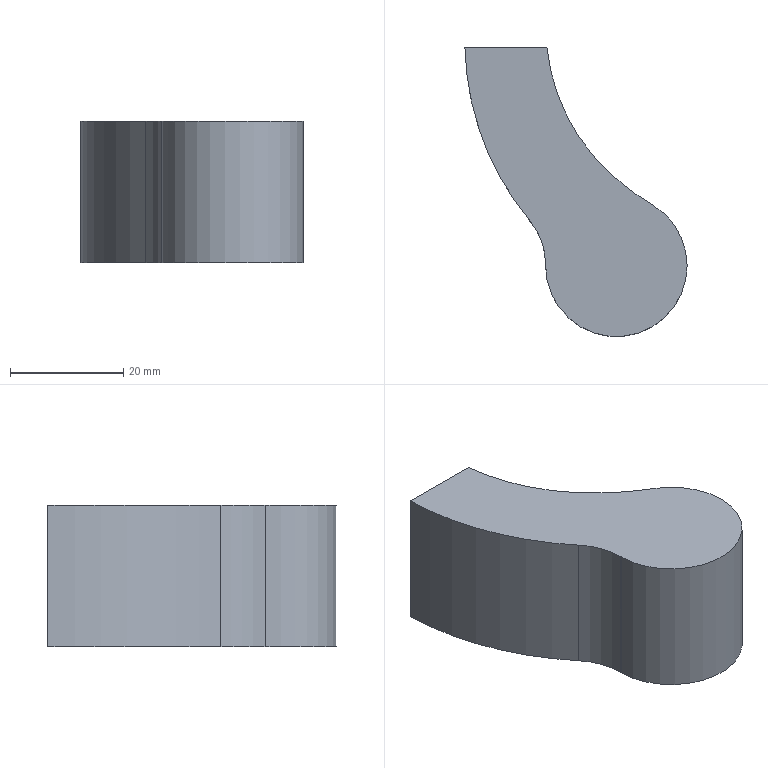Part | SolidWorks | features BaseBody 1 | 1 solid | 19 faces | box 39.25 x 51 x 25 mm | volume 19641 mm3 | cylinder 13 | plane 6 | commonest cylinder face diameters 3.3 x4 25 x3 18 x2 24 x1 70 x1 90 x1
STEP:
#1=CARTESIAN_POINT('',(89.772,84.898,25.));
#2=VERTEX_POINT('',#1);
#3=CARTESIAN_POINT('',(83.667,95.639,25.));
#4=VERTEX_POINT('',#3);
#5=CARTESIAN_POINT('',(77.272,84.898,25.));
#6=DIRECTION('',(0.,0.,1.));
#7=DIRECTION('',(-1.,0.,0.));
#8=AXIS2_PLACEMENT_3D('',#5,#6,#7);
#9=CIRCLE('',#8,12.5);
#10=EDGE_CURVE('',#2,#4,#9,.T.);
#11=ORIENTED_EDGE('',*,*,#10,.F.);
#12=CARTESIAN_POINT('',(89.772,84.898,0.));
#13=VERTEX_POINT('',#12);
#14=CARTESIAN_POINT('',(89.772,84.898,25.));
#15=DIRECTION('',(0.,0.,-1.));
#16=VECTOR('',#15,1000.);
#17=LINE('',#14,#16);
#18=EDGE_CURVE('',#2,#13,#17,.T.);
#19=ORIENTED_EDGE('',*,*,#18,.T.);
#20=CARTESIAN_POINT('',(83.667,95.639,0.));
#21=VERTEX_POINT('',#20);
#22=CARTESIAN_POINT('',(77.272,84.898,0.));
#23=DIRECTION('',(0.,0.,1.));
#24=DIRECTION('',(-1.,0.,0.));
#25=AXIS2_PLACEMENT_3D('',#22,#23,#24);
#26=CIRCLE('',#25,12.5);
#27=EDGE_CURVE('',#13,#21,#26,.T.);
#28=ORIENTED_EDGE('',*,*,#27,.T.);
#29=CARTESIAN_POINT('',(83.667,95.639,25.));
#30=DIRECTION('',(0.,0.,1.));
#31=VECTOR('',#30,1000.);
#32=LINE('',#29,#31);
#33=EDGE_CURVE('',#21,#4,#32,.T.);
#34=ORIENTED_EDGE('',*,*,#33,.T.);
#35=EDGE_LOOP('',(#11,#19,#28,#34));
#36=FACE_OUTER_BOUND('',#35,.T.);
#37=CARTESIAN_POINT('',(77.272,84.898,25.));
#38=DIRECTION('',(0.,0.,-1.));
#39=DIRECTION('',(-1.,0.,0.));
#40=AXIS2_PLACEMENT_3D('',#37,#38,#39);
#41=CYLINDRICAL_SURFACE('',#40,12.5);
#42=ADVANCED_FACE('',(#36),#41,.T.);
#43=ORIENTED_EDGE('',*,*,#18,.F.);
#44=CARTESIAN_POINT('',(64.772,84.898,25.));
#45=VERTEX_POINT('',#44);
#46=CARTESIAN_POINT('',(77.272,84.898,25.));
#47=DIRECTION('',(0.,0.,1.));
#48=DIRECTION('',(-1.,0.,0.));
#49=AXIS2_PLACEMENT_3D('',#46,#47,#48);
#50=CIRCLE('',#49,12.5);
#51=EDGE_CURVE('',#45,#2,#50,.T.);
#52=ORIENTED_EDGE('',*,*,#51,.F.);
#53=CARTESIAN_POINT('',(64.772,84.898,0.));
#54=VERTEX_POINT('',#53);
#55=CARTESIAN_POINT('',(64.772,84.898,25.));
#56=DIRECTION('',(0.,0.,-1.));
#57=VECTOR('',#56,1000.);
#58=LINE('',#55,#57);
#59=EDGE_CURVE('',#45,#54,#58,.T.);
#60=ORIENTED_EDGE('',*,*,#59,.T.);
#61=CARTESIAN_POINT('',(77.272,84.898,0.));
#62=DIRECTION('',(0.,0.,1.));
#63=DIRECTION('',(-1.,0.,0.));
#64=AXIS2_PLACEMENT_3D('',#61,#62,#63);
#65=CIRCLE('',#64,12.5);
#66=EDGE_CURVE('',#54,#13,#65,.T.);
#67=ORIENTED_EDGE('',*,*,#66,.T.);
#68=EDGE_LOOP('',(#43,#52,#60,#67));
#69=FACE_OUTER_BOUND('',#68,.T.);
#70=CARTESIAN_POINT('',(77.272,84.898,25.));
#71=DIRECTION('',(0.,0.,-1.));
#72=DIRECTION('',(-1.,0.,0.));
#73=AXIS2_PLACEMENT_3D('',#70,#71,#72);
#74=CYLINDRICAL_SURFACE('',#73,12.5);
#75=ADVANCED_FACE('',(#69),#74,.T.);
#76=CARTESIAN_POINT('',(59.422,113.398,17.5));
#77=VERTEX_POINT('',#76);
#78=CARTESIAN_POINT('',(56.122,113.398,17.5));
#79=VERTEX_POINT('',#78);
#80=CARTESIAN_POINT('',(57.772,113.398,17.5));
#81=DIRECTION('',(0.,1.,0.));
#82=DIRECTION('',(-1.,0.,0.));
#83=AXIS2_PLACEMENT_3D('',#80,#81,#82);
#84=CIRCLE('',#83,1.65);
#85=EDGE_CURVE('',#77,#79,#84,.T.);
#86=ORIENTED_EDGE('',*,*,#85,.F.);
#87=CARTESIAN_POINT('',(59.422,123.398,17.5));
#88=VERTEX_POINT('',#87);
#89=CARTESIAN_POINT('',(59.422,113.398,17.5));
#90=DIRECTION('',(0.,1.,0.));
#91=VECTOR('',#90,1000.);
#92=LINE('',#89,#91);
#93=EDGE_CURVE('',#77,#88,#92,.T.);
#94=ORIENTED_EDGE('',*,*,#93,.T.);
#95=CARTESIAN_POINT('',(56.122,123.398,17.5));
#96=VERTEX_POINT('',#95);
#97=CARTESIAN_POINT('',(57.772,123.398,17.5));
#98=DIRECTION('',(0.,1.,0.));
#99=DIRECTION('',(-1.,0.,0.));
#100=AXIS2_PLACEMENT_3D('',#97,#98,#99);
#101=CIRCLE('',#100,1.65);
#102=EDGE_CURVE('',#88,#96,#101,.T.);
#103=ORIENTED_EDGE('',*,*,#102,.T.);
#104=CARTESIAN_POINT('',(56.122,113.398,17.5));
#105=DIRECTION('',(0.,1.,0.));
#106=VECTOR('',#105,1000.);
#107=LINE('',#104,#106);
#108=EDGE_CURVE('',#79,#96,#107,.T.);
#109=ORIENTED_EDGE('',*,*,#108,.F.);
#110=EDGE_LOOP('',(#86,#94,#103,#109));
#111=FACE_OUTER_BOUND('',#110,.T.);
#112=CARTESIAN_POINT('',(57.772,113.398,17.5));
#113=DIRECTION('',(0.,1.,0.));
#114=DIRECTION('',(-1.,0.,0.));
#115=AXIS2_PLACEMENT_3D('',#112,#113,#114);
#116=CYLINDRICAL_SURFACE('',#115,1.65);
#117=ADVANCED_FACE('',(#111),#116,.F.);
#118=CARTESIAN_POINT('',(59.422,113.398,7.5));
#119=VERTEX_POINT('',#118);
#120=CARTESIAN_POINT('',(56.122,113.398,7.5));
#121=VERTEX_POINT('',#120);
#122=CARTESIAN_POINT('',(57.772,113.398,7.5));
#123=DIRECTION('',(0.,1.,0.));
#124=DIRECTION('',(-1.,0.,0.));
#125=AXIS2_PLACEMENT_3D('',#122,#123,#124);
#126=CIRCLE('',#125,1.65);
#127=EDGE_CURVE('',#119,#121,#126,.T.);
#128=ORIENTED_EDGE('',*,*,#127,.F.);
#129=CARTESIAN_POINT('',(59.422,123.398,7.5));
#130=VERTEX_POINT('',#129);
#131=CARTESIAN_POINT('',(59.422,113.398,7.5));
#132=DIRECTION('',(0.,1.,0.));
#133=VECTOR('',#132,1000.);
#134=LINE('',#131,#133);
#135=EDGE_CURVE('',#119,#130,#134,.T.);
#136=ORIENTED_EDGE('',*,*,#135,.T.);
#137=CARTESIAN_POINT('',(56.122,123.398,7.5));
#138=VERTEX_POINT('',#137);
#139=CARTESIAN_POINT('',(57.772,123.398,7.5));
#140=DIRECTION('',(0.,1.,0.));
#141=DIRECTION('',(-1.,0.,0.));
#142=AXIS2_PLACEMENT_3D('',#139,#140,#141);
#143=CIRCLE('',#142,1.65);
#144=EDGE_CURVE('',#130,#138,#143,.T.);
#145=ORIENTED_EDGE('',*,*,#144,.T.);
#146=CARTESIAN_POINT('',(56.122,113.398,7.5));
#147=DIRECTION('',(0.,1.,0.));
#148=VECTOR('',#147,1000.);
#149=LINE('',#146,#148);
#150=EDGE_CURVE('',#121,#138,#149,.T.);
#151=ORIENTED_EDGE('',*,*,#150,.F.);
#152=EDGE_LOOP('',(#128,#136,#145,#151));
#153=FACE_OUTER_BOUND('',#152,.T.);
#154=CARTESIAN_POINT('',(57.772,113.398,7.5));
#155=DIRECTION('',(0.,1.,0.));
#156=DIRECTION('',(-1.,0.,0.));
#157=AXIS2_PLACEMENT_3D('',#154,#155,#156);
#158=CYLINDRICAL_SURFACE('',#157,1.65);
#159=ADVANCED_FACE('',(#153),#158,.F.);
#160=CARTESIAN_POINT('',(86.272,84.898,20.));
#161=VERTEX_POINT('',#160);
#162=CARTESIAN_POINT('',(68.272,84.898,20.));
#163=VERTEX_POINT('',#162);
#164=CARTESIAN_POINT('',(77.272,84.898,20.));
#165=DIRECTION('',(0.,0.,-1.));
#166=DIRECTION('',(-1.,0.,0.));
#167=AXIS2_PLACEMENT_3D('',#164,#165,#166);
#168=CIRCLE('',#167,9.);
#169=EDGE_CURVE('',#161,#163,#168,.T.);
#170=ORIENTED_EDGE('',*,*,#169,.F.);
#171=CARTESIAN_POINT('',(86.272,84.898,0.));
#172=VERTEX_POINT('',#171);
#173=CARTESIAN_POINT('',(86.272,84.898,20.));
#174=DIRECTION('',(0.,0.,-1.));
#175=VECTOR('',#174,1000.);
#176=LINE('',#173,#175);
#177=EDGE_CURVE('',#161,#172,#176,.T.);
#178=ORIENTED_EDGE('',*,*,#177,.T.);
#179=CARTESIAN_POINT('',(68.272,84.898,0.));
#180=VERTEX_POINT('',#179);
#181=CARTESIAN_POINT('',(77.272,84.898,0.));
#182=DIRECTION('',(0.,0.,-1.));
#183=DIRECTION('',(-1.,0.,0.));
#184=AXIS2_PLACEMENT_3D('',#181,#182,#183);
#185=CIRCLE('',#184,9.);
#186=EDGE_CURVE('',#172,#180,#185,.T.);
#187=ORIENTED_EDGE('',*,*,#186,.T.);
#188=CARTESIAN_POINT('',(68.272,84.898,20.));
#189=DIRECTION('',(0.,0.,-1.));
#190=VECTOR('',#189,1000.);
#191=LINE('',#188,#190);
#192=EDGE_CURVE('',#163,#180,#191,.T.);
#193=ORIENTED_EDGE('',*,*,#192,.F.);
#194=EDGE_LOOP('',(#170,#178,#187,#193));
#195=FACE_OUTER_BOUND('',#194,.T.);
#196=CARTESIAN_POINT('',(77.272,84.898,20.));
#197=DIRECTION('',(0.,0.,-1.));
#198=DIRECTION('',(-1.,0.,0.));
#199=AXIS2_PLACEMENT_3D('',#196,#197,#198);
#200=CYLINDRICAL_SURFACE('',#199,9.);
#201=ADVANCED_FACE('',(#195),#200,.F.);
#202=CARTESIAN_POINT('',(64.773,85.034,25.));
#203=VERTEX_POINT('',#202);
#204=CARTESIAN_POINT('',(77.272,84.898,25.));
#205=DIRECTION('',(0.,0.,1.));
#206=DIRECTION('',(-1.,0.,0.));
#207=AXIS2_PLACEMENT_3D('',#204,#205,#206);
#208=CIRCLE('',#207,12.5);
#209=EDGE_CURVE('',#203,#45,#208,.T.);
#210=ORIENTED_EDGE('',*,*,#209,.T.);
#211=ORIENTED_EDGE('',*,*,#51,.T.);
#212=ORIENTED_EDGE('',*,*,#10,.T.);
#213=CARTESIAN_POINT('',(75.841,101.541,25.));
#214=VERTEX_POINT('',#213);
#215=CARTESIAN_POINT('',(106.689,134.304,25.));
#216=DIRECTION('',(0.,0.,-1.));
#217=DIRECTION('',(-1.,0.,0.));
#218=AXIS2_PLACEMENT_3D('',#215,#216,#217);
#219=CIRCLE('',#218,45.);
#220=EDGE_CURVE('',#4,#214,#219,.T.);
#221=ORIENTED_EDGE('',*,*,#220,.T.);
#222=CARTESIAN_POINT('',(65.022,123.398,25.));
#223=VERTEX_POINT('',#222);
#224=CARTESIAN_POINT('',(99.834,127.023,25.));
#225=DIRECTION('',(0.,0.,-1.));
#226=DIRECTION('',(-1.,0.,0.));
#227=AXIS2_PLACEMENT_3D('',#224,#225,#226);
#228=CIRCLE('',#227,35.);
#229=EDGE_CURVE('',#214,#223,#228,.T.);
#230=ORIENTED_EDGE('',*,*,#229,.T.);
#231=CARTESIAN_POINT('',(50.522,123.398,25.));
#232=VERTEX_POINT('',#231);
#233=CARTESIAN_POINT('',(99.834,123.398,25.));
#234=DIRECTION('',(-1.,0.,0.));
#235=VECTOR('',#234,1000.);
#236=LINE('',#233,#235);
#237=EDGE_CURVE('',#223,#232,#236,.T.);
#238=ORIENTED_EDGE('',*,*,#237,.T.);
#239=CARTESIAN_POINT('',(62.011,92.823,25.));
#240=VERTEX_POINT('',#239);
#241=CARTESIAN_POINT('',(100.504,124.734,25.));
#242=DIRECTION('',(0.,0.,1.));
#243=DIRECTION('',(-1.,0.,0.));
#244=AXIS2_PLACEMENT_3D('',#241,#242,#243);
#245=CIRCLE('',#244,50.);
#246=EDGE_CURVE('',#232,#240,#245,.T.);
#247=ORIENTED_EDGE('',*,*,#246,.T.);
#248=CARTESIAN_POINT('',(52.773,85.164,25.));
#249=DIRECTION('',(0.,0.,-1.));
#250=DIRECTION('',(-1.,0.,0.));
#251=AXIS2_PLACEMENT_3D('',#248,#249,#250);
#252=CIRCLE('',#251,12.);
#253=EDGE_CURVE('',#240,#203,#252,.T.);
#254=ORIENTED_EDGE('',*,*,#253,.T.);
#255=EDGE_LOOP('',(#210,#211,#212,#221,#230,#238,#247,#254));
#256=FACE_OUTER_BOUND('',#255,.T.);
#257=CARTESIAN_POINT('',(99.834,127.023,25.));
#258=DIRECTION('',(0.,0.,1.));
#259=DIRECTION('',(1.,0.,0.));
#260=AXIS2_PLACEMENT_3D('',#257,#258,#259);
#261=PLANE('',#260);
#262=ADVANCED_FACE('',(#256),#261,.T.);
#263=CARTESIAN_POINT('',(75.841,101.541,0.));
#264=VERTEX_POINT('',#263);
#265=CARTESIAN_POINT('',(75.841,101.541,25.));
#266=DIRECTION('',(0.,0.,-1.));
#267=VECTOR('',#266,1000.);
#268=LINE('',#265,#267);
#269=EDGE_CURVE('',#214,#264,#268,.T.);
#270=ORIENTED_EDGE('',*,*,#269,.F.);
#271=ORIENTED_EDGE('',*,*,#220,.F.);
#272=ORIENTED_EDGE('',*,*,#33,.F.);
#273=CARTESIAN_POINT('',(106.689,134.304,0.));
#274=DIRECTION('',(0.,0.,1.));
#275=DIRECTION('',(-1.,0.,0.));
#276=AXIS2_PLACEMENT_3D('',#273,#274,#275);
#277=CIRCLE('',#276,45.);
#278=EDGE_CURVE('',#264,#21,#277,.T.);
#279=ORIENTED_EDGE('',*,*,#278,.F.);
#280=EDGE_LOOP('',(#270,#271,#272,#279));
#281=FACE_OUTER_BOUND('',#280,.T.);
#282=CARTESIAN_POINT('',(106.689,134.304,25.));
#283=DIRECTION('',(0.,0.,-1.));
#284=DIRECTION('',(-1.,0.,0.));
#285=AXIS2_PLACEMENT_3D('',#282,#283,#284);
#286=CYLINDRICAL_SURFACE('',#285,45.);
#287=ADVANCED_FACE('',(#281),#286,.F.);
#288=ORIENTED_EDGE('',*,*,#59,.F.);
#289=ORIENTED_EDGE('',*,*,#209,.F.);
#290=CARTESIAN_POINT('',(64.773,85.034,0.));
#291=VERTEX_POINT('',#290);
#292=CARTESIAN_POINT('',(64.773,85.034,25.));
#293=DIRECTION('',(0.,0.,-1.));
#294=VECTOR('',#293,1000.);
#295=LINE('',#292,#294);
#296=EDGE_CURVE('',#203,#291,#295,.T.);
#297=ORIENTED_EDGE('',*,*,#296,.T.);
#298=CARTESIAN_POINT('',(77.272,84.898,0.));
#299=DIRECTION('',(0.,0.,1.));
#300=DIRECTION('',(-1.,0.,0.));
#301=AXIS2_PLACEMENT_3D('',#298,#299,#300);
#302=CIRCLE('',#301,12.5);
#303=EDGE_CURVE('',#291,#54,#302,.T.);
#304=ORIENTED_EDGE('',*,*,#303,.T.);
#305=EDGE_LOOP('',(#288,#289,#297,#304));
#306=FACE_OUTER_BOUND('',#305,.T.);
#307=CARTESIAN_POINT('',(77.272,84.898,25.));
#308=DIRECTION('',(0.,0.,-1.));
#309=DIRECTION('',(-1.,0.,0.));
#310=AXIS2_PLACEMENT_3D('',#307,#308,#309);
#311=CYLINDRICAL_SURFACE('',#310,12.5);
#312=ADVANCED_FACE('',(#306),#311,.T.);
#313=ORIENTED_EDGE('',*,*,#296,.F.);
#314=ORIENTED_EDGE('',*,*,#253,.F.);
#315=CARTESIAN_POINT('',(62.011,92.823,0.));
#316=VERTEX_POINT('',#315);
#317=CARTESIAN_POINT('',(62.011,92.823,25.));
#318=DIRECTION('',(0.,0.,1.));
#319=VECTOR('',#318,1000.);
#320=LINE('',#317,#319);
#321=EDGE_CURVE('',#316,#240,#320,.T.);
#322=ORIENTED_EDGE('',*,*,#321,.F.);
#323=CARTESIAN_POINT('',(52.773,85.164,0.));
#324=DIRECTION('',(0.,0.,1.));
#325=DIRECTION('',(-1.,0.,0.));
#326=AXIS2_PLACEMENT_3D('',#323,#324,#325);
#327=CIRCLE('',#326,12.);
#328=EDGE_CURVE('',#291,#316,#327,.T.);
#329=ORIENTED_EDGE('',*,*,#328,.F.);
#330=EDGE_LOOP('',(#313,#314,#322,#329));
#331=FACE_OUTER_BOUND('',#330,.T.);
#332=CARTESIAN_POINT('',(52.773,85.164,25.));
#333=DIRECTION('',(0.,0.,-1.));
#334=DIRECTION('',(-1.,0.,0.));
#335=AXIS2_PLACEMENT_3D('',#332,#333,#334);
#336=CYLINDRICAL_SURFACE('',#335,12.);
#337=ADVANCED_FACE('',(#331),#336,.F.);
#338=ORIENTED_EDGE('',*,*,#246,.F.);
#339=CARTESIAN_POINT('',(50.522,123.398,0.));
#340=VERTEX_POINT('',#339);
#341=CARTESIAN_POINT('',(50.522,123.398,25.));
#342=DIRECTION('',(0.,0.,-1.));
#343=VECTOR('',#342,1000.);
#344=LINE('',#341,#343);
#345=EDGE_CURVE('',#232,#340,#344,.T.);
#346=ORIENTED_EDGE('',*,*,#345,.T.);
#347=CARTESIAN_POINT('',(100.504,124.734,0.));
#348=DIRECTION('',(0.,0.,1.));
#349=DIRECTION('',(-1.,0.,0.));
#350=AXIS2_PLACEMENT_3D('',#347,#348,#349);
#351=CIRCLE('',#350,50.);
#352=EDGE_CURVE('',#340,#316,#351,.T.);
#353=ORIENTED_EDGE('',*,*,#352,.T.);
#354=ORIENTED_EDGE('',*,*,#321,.T.);
#355=EDGE_LOOP('',(#338,#346,#353,#354));
#356=FACE_OUTER_BOUND('',#355,.T.);
#357=CARTESIAN_POINT('',(100.504,124.734,25.));
#358=DIRECTION('',(0.,0.,-1.));
#359=DIRECTION('',(-1.,0.,0.));
#360=AXIS2_PLACEMENT_3D('',#357,#358,#359);
#361=CYLINDRICAL_SURFACE('',#360,50.);
#362=ADVANCED_FACE('',(#356),#361,.T.);
#363=ORIENTED_EDGE('',*,*,#345,.F.);
#364=ORIENTED_EDGE('',*,*,#237,.F.);
#365=CARTESIAN_POINT('',(65.022,123.398,0.));
#366=VERTEX_POINT('',#365);
#367=CARTESIAN_POINT('',(65.022,123.398,25.));
#368=DIRECTION('',(0.,0.,1.));
#369=VECTOR('',#368,1000.);
#370=LINE('',#367,#369);
#371=EDGE_CURVE('',#366,#223,#370,.T.);
#372=ORIENTED_EDGE('',*,*,#371,.F.);
#373=CARTESIAN_POINT('',(65.022,123.398,0.));
#374=DIRECTION('',(1.,0.,0.));
#375=VECTOR('',#374,1000.);
#376=LINE('',#373,#375);
#377=EDGE_CURVE('',#340,#366,#376,.T.);
#378=ORIENTED_EDGE('',*,*,#377,.F.);
#379=EDGE_LOOP('',(#363,#364,#372,#378));
#380=FACE_OUTER_BOUND('',#379,.T.);
#381=CARTESIAN_POINT('',(57.772,123.398,17.5));
#382=DIRECTION('',(0.,1.,0.));
#383=DIRECTION('',(-1.,0.,0.));
#384=AXIS2_PLACEMENT_3D('',#381,#382,#383);
#385=CIRCLE('',#384,1.65);
#386=EDGE_CURVE('',#96,#88,#385,.T.);
#387=ORIENTED_EDGE('',*,*,#386,.F.);
#388=ORIENTED_EDGE('',*,*,#102,.F.);
#389=EDGE_LOOP('',(#387,#388));
#390=FACE_BOUND('',#389,.T.);
#391=CARTESIAN_POINT('',(57.772,123.398,7.5));
#392=DIRECTION('',(0.,1.,0.));
#393=DIRECTION('',(-1.,0.,0.));
#394=AXIS2_PLACEMENT_3D('',#391,#392,#393);
#395=CIRCLE('',#394,1.65);
#396=EDGE_CURVE('',#138,#130,#395,.T.);
#397=ORIENTED_EDGE('',*,*,#396,.F.);
#398=ORIENTED_EDGE('',*,*,#144,.F.);
#399=EDGE_LOOP('',(#397,#398));
#400=FACE_BOUND('',#399,.T.);
#401=CARTESIAN_POINT('',(65.022,123.398,25.));
#402=DIRECTION('',(0.,-1.,0.));
#403=DIRECTION('',(1.,0.,0.));
#404=AXIS2_PLACEMENT_3D('',#401,#402,#403);
#405=PLANE('',#404);
#406=ADVANCED_FACE('',(#380,#390,#400),#405,.F.);
#407=ORIENTED_EDGE('',*,*,#371,.T.);
#408=ORIENTED_EDGE('',*,*,#229,.F.);
#409=ORIENTED_EDGE('',*,*,#269,.T.);
#410=CARTESIAN_POINT('',(99.834,127.023,0.));
#411=DIRECTION('',(0.,0.,1.));
#412=DIRECTION('',(-1.,0.,0.));
#413=AXIS2_PLACEMENT_3D('',#410,#411,#412);
#414=CIRCLE('',#413,35.);
#415=EDGE_CURVE('',#366,#264,#414,.T.);
#416=ORIENTED_EDGE('',*,*,#415,.F.);
#417=EDGE_LOOP('',(#407,#408,#409,#416));
#418=FACE_OUTER_BOUND('',#417,.T.);
#419=CARTESIAN_POINT('',(99.834,127.023,25.));
#420=DIRECTION('',(0.,0.,-1.));
#421=DIRECTION('',(-1.,0.,0.));
#422=AXIS2_PLACEMENT_3D('',#419,#420,#421);
#423=CYLINDRICAL_SURFACE('',#422,35.);
#424=ADVANCED_FACE('',(#418),#423,.F.);
#425=ORIENTED_EDGE('',*,*,#278,.T.);
#426=ORIENTED_EDGE('',*,*,#27,.F.);
#427=ORIENTED_EDGE('',*,*,#66,.F.);
#428=ORIENTED_EDGE('',*,*,#303,.F.);
#429=ORIENTED_EDGE('',*,*,#328,.T.);
#430=ORIENTED_EDGE('',*,*,#352,.F.);
#431=ORIENTED_EDGE('',*,*,#377,.T.);
#432=ORIENTED_EDGE('',*,*,#415,.T.);
#433=EDGE_LOOP('',(#425,#426,#427,#428,#429,#430,#431,#432));
#434=FACE_OUTER_BOUND('',#433,.T.);
#435=CARTESIAN_POINT('',(77.272,84.898,0.));
#436=DIRECTION('',(0.,0.,-1.));
#437=DIRECTION('',(-1.,0.,0.));
#438=AXIS2_PLACEMENT_3D('',#435,#436,#437);
#439=CIRCLE('',#438,9.);
#440=EDGE_CURVE('',#180,#172,#439,.T.);
#441=ORIENTED_EDGE('',*,*,#440,.F.);
#442=ORIENTED_EDGE('',*,*,#186,.F.);
#443=EDGE_LOOP('',(#441,#442));
#444=FACE_BOUND('',#443,.T.);
#445=CARTESIAN_POINT('',(99.834,127.023,0.));
#446=DIRECTION('',(0.,0.,1.));
#447=DIRECTION('',(1.,0.,0.));
#448=AXIS2_PLACEMENT_3D('',#445,#446,#447);
#449=PLANE('',#448);
#450=ADVANCED_FACE('',(#434,#444),#449,.F.);
#451=ORIENTED_EDGE('',*,*,#93,.F.);
#452=CARTESIAN_POINT('',(57.772,113.398,17.5));
#453=DIRECTION('',(0.,1.,0.));
#454=DIRECTION('',(-1.,0.,0.));
#455=AXIS2_PLACEMENT_3D('',#452,#453,#454);
#456=CIRCLE('',#455,1.65);
#457=EDGE_CURVE('',#79,#77,#456,.T.);
#458=ORIENTED_EDGE('',*,*,#457,.F.);
#459=ORIENTED_EDGE('',*,*,#108,.T.);
#460=ORIENTED_EDGE('',*,*,#386,.T.);
#461=EDGE_LOOP('',(#451,#458,#459,#460));
#462=FACE_OUTER_BOUND('',#461,.T.);
#463=CARTESIAN_POINT('',(57.772,113.398,17.5));
#464=DIRECTION('',(0.,1.,0.));
#465=DIRECTION('',(-1.,0.,0.));
#466=AXIS2_PLACEMENT_3D('',#463,#464,#465);
#467=CYLINDRICAL_SURFACE('',#466,1.65);
#468=ADVANCED_FACE('',(#462),#467,.F.);
#469=ORIENTED_EDGE('',*,*,#135,.F.);
#470=CARTESIAN_POINT('',(57.772,113.398,7.5));
#471=DIRECTION('',(0.,1.,0.));
#472=DIRECTION('',(-1.,0.,0.));
#473=AXIS2_PLACEMENT_3D('',#470,#471,#472);
#474=CIRCLE('',#473,1.65);
#475=EDGE_CURVE('',#121,#119,#474,.T.);
#476=ORIENTED_EDGE('',*,*,#475,.F.);
#477=ORIENTED_EDGE('',*,*,#150,.T.);
#478=ORIENTED_EDGE('',*,*,#396,.T.);
#479=EDGE_LOOP('',(#469,#476,#477,#478));
#480=FACE_OUTER_BOUND('',#479,.T.);
#481=CARTESIAN_POINT('',(57.772,113.398,7.5));
#482=DIRECTION('',(0.,1.,0.));
#483=DIRECTION('',(-1.,0.,0.));
#484=AXIS2_PLACEMENT_3D('',#481,#482,#483);
#485=CYLINDRICAL_SURFACE('',#484,1.65);
#486=ADVANCED_FACE('',(#480),#485,.F.);
#487=ORIENTED_EDGE('',*,*,#177,.F.);
#488=CARTESIAN_POINT('',(77.272,84.898,20.));
#489=DIRECTION('',(0.,0.,-1.));
#490=DIRECTION('',(-1.,0.,0.));
#491=AXIS2_PLACEMENT_3D('',#488,#489,#490);
#492=CIRCLE('',#491,9.);
#493=EDGE_CURVE('',#163,#161,#492,.T.);
#494=ORIENTED_EDGE('',*,*,#493,.F.);
#495=ORIENTED_EDGE('',*,*,#192,.T.);
#496=ORIENTED_EDGE('',*,*,#440,.T.);
#497=EDGE_LOOP('',(#487,#494,#495,#496));
#498=FACE_OUTER_BOUND('',#497,.T.);
#499=CARTESIAN_POINT('',(77.272,84.898,20.));
#500=DIRECTION('',(0.,0.,-1.));
#501=DIRECTION('',(-1.,0.,0.));
#502=AXIS2_PLACEMENT_3D('',#499,#500,#501);
#503=CYLINDRICAL_SURFACE('',#502,9.);
#504=ADVANCED_FACE('',(#498),#503,.F.);
#505=ORIENTED_EDGE('',*,*,#457,.T.);
#506=ORIENTED_EDGE('',*,*,#85,.T.);
#507=EDGE_LOOP('',(#505,#506));
#508=FACE_OUTER_BOUND('',#507,.T.);
#509=CARTESIAN_POINT('',(57.772,113.398,17.5));
#510=DIRECTION('',(0.,1.,0.));
#511=DIRECTION('',(-1.,0.,0.));
#512=AXIS2_PLACEMENT_3D('',#509,#510,#511);
#513=PLANE('',#512);
#514=ADVANCED_FACE('',(#508),#513,.T.);
#515=ORIENTED_EDGE('',*,*,#475,.T.);
#516=ORIENTED_EDGE('',*,*,#127,.T.);
#517=EDGE_LOOP('',(#515,#516));
#518=FACE_OUTER_BOUND('',#517,.T.);
#519=CARTESIAN_POINT('',(57.772,113.398,7.5));
#520=DIRECTION('',(0.,1.,0.));
#521=DIRECTION('',(-1.,0.,0.));
#522=AXIS2_PLACEMENT_3D('',#519,#520,#521);
#523=PLANE('',#522);
#524=ADVANCED_FACE('',(#518),#523,.T.);
#525=ORIENTED_EDGE('',*,*,#493,.T.);
#526=ORIENTED_EDGE('',*,*,#169,.T.);
#527=EDGE_LOOP('',(#525,#526));
#528=FACE_OUTER_BOUND('',#527,.T.);
#529=CARTESIAN_POINT('',(77.272,84.898,20.));
#530=DIRECTION('',(0.,0.,-1.));
#531=DIRECTION('',(-1.,0.,0.));
#532=AXIS2_PLACEMENT_3D('',#529,#530,#531);
#533=PLANE('',#532);
#534=ADVANCED_FACE('',(#528),#533,.T.);
#535=CLOSED_SHELL('',(#42,#75,#117,#159,#201,#262,#287,#312,#337,#362,#406,#424,#450,#468,#486,#504,#514,#524,#534));
#536=MANIFOLD_SOLID_BREP('',#535);
#537=CARTESIAN_POINT('',(0.,0.,0.));
#538=DIRECTION('',(0.,0.,1.));
#539=DIRECTION('',(1.,0.,0.));
#540=AXIS2_PLACEMENT_3D('',#537,#538,#539);
#541=(LENGTH_UNIT()NAMED_UNIT(*)SI_UNIT(.MILLI.,.METRE.));
#542=UNCERTAINTY_MEASURE_WITH_UNIT(LENGTH_MEASURE(0.00001),#541,'','');
#543=(NAMED_UNIT(*)PLANE_ANGLE_UNIT()SI_UNIT($,.RADIAN.));
#544=(NAMED_UNIT(*)SI_UNIT($,.STERADIAN.)SOLID_ANGLE_UNIT());
#545=(GEOMETRIC_REPRESENTATION_CONTEXT(3)GLOBAL_UNCERTAINTY_ASSIGNED_CONTEXT((#542))GLOBAL_UNIT_ASSIGNED_CONTEXT((#541,#543,#544))REPRESENTATION_CONTEXT('',''));
#546=ADVANCED_BREP_SHAPE_REPRESENTATION('',(#536,#540),#545);